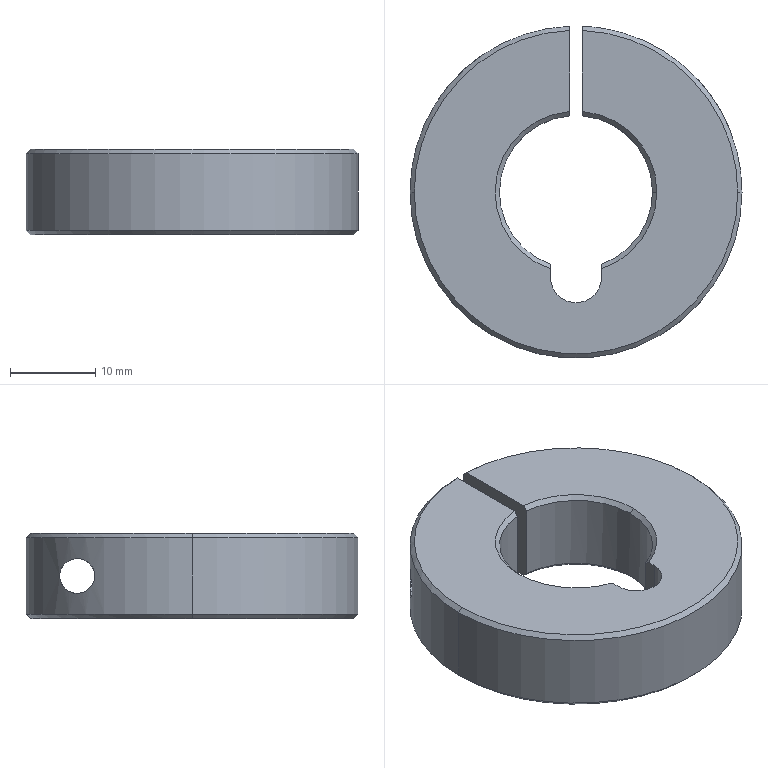Part | SolidWorks | features BaseBody 1 | 1 solid | 40 faces | box 39 x 38.986 x 10 mm | volume 8129 mm3 | cone 16 | cylinder 15 | plane 9 | commonest cylinder face diameters 5.5 x4 39 x4 18 x3 4.1 x2 6 x1 9 x1
STEP:
#1=CARTESIAN_POINT('',(5.,13.5,-2.75));
#2=VERTEX_POINT('',#1);
#3=CARTESIAN_POINT('',(5.,13.5,2.75));
#4=VERTEX_POINT('',#3);
#5=CARTESIAN_POINT('',(5.,13.5,0.));
#6=DIRECTION('',(-1.,0.,0.));
#7=DIRECTION('',(0.,0.,1.));
#8=AXIS2_PLACEMENT_3D('',#5,#6,#7);
#9=CIRCLE('',#8,2.75);
#10=EDGE_CURVE('',#2,#4,#9,.T.);
#11=ORIENTED_EDGE('',*,*,#10,.T.);
#12=CARTESIAN_POINT('',(5.5,13.5,3.25));
#13=VERTEX_POINT('',#12);
#14=CARTESIAN_POINT('',(5.5,13.5,3.25));
#15=DIRECTION('',(0.7071,0.,0.7071));
#16=VECTOR('',#15,1000.);
#17=LINE('',#14,#16);
#18=EDGE_CURVE('',#4,#13,#17,.T.);
#19=ORIENTED_EDGE('',*,*,#18,.T.);
#20=CARTESIAN_POINT('',(5.5,13.5,-3.25));
#21=VERTEX_POINT('',#20);
#22=CARTESIAN_POINT('',(5.5,13.5,0.));
#23=DIRECTION('',(-1.,0.,0.));
#24=DIRECTION('',(0.,0.,1.));
#25=AXIS2_PLACEMENT_3D('',#22,#23,#24);
#26=CIRCLE('',#25,3.25);
#27=EDGE_CURVE('',#21,#13,#26,.T.);
#28=ORIENTED_EDGE('',*,*,#27,.F.);
#29=CARTESIAN_POINT('',(5.5,13.5,-3.25));
#30=DIRECTION('',(0.7071,0.,-0.7071));
#31=VECTOR('',#30,1000.);
#32=LINE('',#29,#31);
#33=EDGE_CURVE('',#2,#21,#32,.T.);
#34=ORIENTED_EDGE('',*,*,#33,.F.);
#35=EDGE_LOOP('',(#11,#19,#28,#34));
#36=FACE_OUTER_BOUND('',#35,.T.);
#37=CARTESIAN_POINT('',(5.5,13.5,0.));
#38=DIRECTION('',(1.,0.,0.));
#39=DIRECTION('',(0.,0.,-1.));
#40=AXIS2_PLACEMENT_3D('',#37,#38,#39);
#41=CONICAL_SURFACE('',#40,3.25,0.7854);
#42=ADVANCED_FACE('',(#36),#41,.F.);
#43=ORIENTED_EDGE('',*,*,#10,.F.);
#44=CARTESIAN_POINT('',(0.75,13.5,-2.75));
#45=VERTEX_POINT('',#44);
#46=CARTESIAN_POINT('',(-35.723,13.5,-2.75));
#47=DIRECTION('',(-1.,0.,0.));
#48=VECTOR('',#47,1000.);
#49=LINE('',#46,#48);
#50=EDGE_CURVE('',#2,#45,#49,.T.);
#51=ORIENTED_EDGE('',*,*,#50,.T.);
#52=CARTESIAN_POINT('',(0.75,13.5,2.75));
#53=VERTEX_POINT('',#52);
#54=CARTESIAN_POINT('',(0.75,13.5,0.));
#55=DIRECTION('',(-1.,0.,0.));
#56=DIRECTION('',(0.,0.,-1.));
#57=AXIS2_PLACEMENT_3D('',#54,#55,#56);
#58=CIRCLE('',#57,2.75);
#59=EDGE_CURVE('',#45,#53,#58,.T.);
#60=ORIENTED_EDGE('',*,*,#59,.T.);
#61=CARTESIAN_POINT('',(-35.723,13.5,2.75));
#62=DIRECTION('',(-1.,0.,0.));
#63=VECTOR('',#62,1000.);
#64=LINE('',#61,#63);
#65=EDGE_CURVE('',#4,#53,#64,.T.);
#66=ORIENTED_EDGE('',*,*,#65,.F.);
#67=EDGE_LOOP('',(#43,#51,#60,#66));
#68=FACE_OUTER_BOUND('',#67,.T.);
#69=CARTESIAN_POINT('',(-35.723,13.5,0.));
#70=DIRECTION('',(-1.,0.,0.));
#71=DIRECTION('',(0.,0.,1.));
#72=AXIS2_PLACEMENT_3D('',#69,#70,#71);
#73=CYLINDRICAL_SURFACE('',#72,2.75);
#74=ADVANCED_FACE('',(#68),#73,.F.);
#75=CARTESIAN_POINT('',(-0.75,13.5,2.75));
#76=VERTEX_POINT('',#75);
#77=CARTESIAN_POINT('',(-0.75,13.5,-2.75));
#78=VERTEX_POINT('',#77);
#79=CARTESIAN_POINT('',(-0.75,13.5,0.));
#80=DIRECTION('',(1.,0.,0.));
#81=DIRECTION('',(0.,0.,1.));
#82=AXIS2_PLACEMENT_3D('',#79,#80,#81);
#83=CIRCLE('',#82,2.75);
#84=EDGE_CURVE('',#76,#78,#83,.T.);
#85=ORIENTED_EDGE('',*,*,#84,.T.);
#86=CARTESIAN_POINT('',(-1.25,13.5,-2.75));
#87=VERTEX_POINT('',#86);
#88=CARTESIAN_POINT('',(-35.723,13.5,-2.75));
#89=DIRECTION('',(-1.,0.,0.));
#90=VECTOR('',#89,1000.);
#91=LINE('',#88,#90);
#92=EDGE_CURVE('',#78,#87,#91,.T.);
#93=ORIENTED_EDGE('',*,*,#92,.T.);
#94=CARTESIAN_POINT('',(-1.25,13.5,2.75));
#95=VERTEX_POINT('',#94);
#96=CARTESIAN_POINT('',(-1.25,13.5,0.));
#97=DIRECTION('',(-1.,0.,0.));
#98=DIRECTION('',(0.,0.,1.));
#99=AXIS2_PLACEMENT_3D('',#96,#97,#98);
#100=CIRCLE('',#99,2.75);
#101=EDGE_CURVE('',#87,#95,#100,.T.);
#102=ORIENTED_EDGE('',*,*,#101,.T.);
#103=CARTESIAN_POINT('',(-35.723,13.5,2.75));
#104=DIRECTION('',(-1.,0.,0.));
#105=VECTOR('',#104,1000.);
#106=LINE('',#103,#105);
#107=EDGE_CURVE('',#76,#95,#106,.T.);
#108=ORIENTED_EDGE('',*,*,#107,.F.);
#109=EDGE_LOOP('',(#85,#93,#102,#108));
#110=FACE_OUTER_BOUND('',#109,.T.);
#111=CARTESIAN_POINT('',(-35.723,13.5,0.));
#112=DIRECTION('',(-1.,0.,0.));
#113=DIRECTION('',(0.,0.,1.));
#114=AXIS2_PLACEMENT_3D('',#111,#112,#113);
#115=CYLINDRICAL_SURFACE('',#114,2.75);
#116=ADVANCED_FACE('',(#110),#115,.F.);
#117=CARTESIAN_POINT('',(-1.654,13.5,-2.05));
#118=VERTEX_POINT('',#117);
#119=CARTESIAN_POINT('',(-1.654,13.5,2.05));
#120=VERTEX_POINT('',#119);
#121=CARTESIAN_POINT('',(-1.654,13.5,0.));
#122=DIRECTION('',(-1.,0.,0.));
#123=DIRECTION('',(0.,0.,1.));
#124=AXIS2_PLACEMENT_3D('',#121,#122,#123);
#125=CIRCLE('',#124,2.05);
#126=EDGE_CURVE('',#118,#120,#125,.T.);
#127=ORIENTED_EDGE('',*,*,#126,.T.);
#128=CARTESIAN_POINT('',(-1.25,13.5,2.75));
#129=DIRECTION('',(0.5,0.,0.866));
#130=VECTOR('',#129,1000.);
#131=LINE('',#128,#130);
#132=EDGE_CURVE('',#120,#95,#131,.T.);
#133=ORIENTED_EDGE('',*,*,#132,.T.);
#134=ORIENTED_EDGE('',*,*,#101,.F.);
#135=CARTESIAN_POINT('',(-1.25,13.5,-2.75));
#136=DIRECTION('',(0.5,0.,-0.866));
#137=VECTOR('',#136,1000.);
#138=LINE('',#135,#137);
#139=EDGE_CURVE('',#118,#87,#138,.T.);
#140=ORIENTED_EDGE('',*,*,#139,.F.);
#141=EDGE_LOOP('',(#127,#133,#134,#140));
#142=FACE_OUTER_BOUND('',#141,.T.);
#143=CARTESIAN_POINT('',(-1.25,13.5,0.));
#144=DIRECTION('',(1.,0.,0.));
#145=DIRECTION('',(0.,0.,-1.));
#146=AXIS2_PLACEMENT_3D('',#143,#144,#145);
#147=CONICAL_SURFACE('',#146,2.75,1.047);
#148=ADVANCED_FACE('',(#142),#147,.F.);
#149=ORIENTED_EDGE('',*,*,#126,.F.);
#150=CARTESIAN_POINT('',(-14.071,13.5,-2.05));
#151=VERTEX_POINT('',#150);
#152=CARTESIAN_POINT('',(-35.723,13.5,-2.05));
#153=DIRECTION('',(-1.,0.,0.));
#154=VECTOR('',#153,1000.);
#155=LINE('',#152,#154);
#156=EDGE_CURVE('',#118,#151,#155,.T.);
#157=ORIENTED_EDGE('',*,*,#156,.T.);
#158=CARTESIAN_POINT('',(-14.071,13.5,2.05));
#159=VERTEX_POINT('',#158);
#160=CARTESIAN_POINT('',(-14.071,13.5,-2.05));
#161=CARTESIAN_POINT('',(-14.193,13.374,-2.05));
#162=CARTESIAN_POINT('',(-14.305,13.253,-2.038));
#163=CARTESIAN_POINT('',(-14.461,13.082,-2.008));
#164=CARTESIAN_POINT('',(-14.51,13.027,-1.995));
#165=CARTESIAN_POINT('',(-14.581,12.947,-1.974));
#166=CARTESIAN_POINT('',(-14.616,12.908,-1.963));
#167=CARTESIAN_POINT('',(-14.655,12.864,-1.949));
#168=CARTESIAN_POINT('',(-14.672,12.845,-1.942));
#169=CARTESIAN_POINT('',(-14.683,12.832,-1.938));
#170=CARTESIAN_POINT('',(-14.687,12.828,-1.937));
#171=CARTESIAN_POINT('',(-14.801,12.696,-1.89));
#172=CARTESIAN_POINT('',(-14.901,12.579,-1.836));
#173=CARTESIAN_POINT('',(-15.037,12.415,-1.741));
#174=CARTESIAN_POINT('',(-15.08,12.363,-1.707));
#175=CARTESIAN_POINT('',(-15.142,12.287,-1.653));
#176=CARTESIAN_POINT('',(-15.172,12.25,-1.625));
#177=CARTESIAN_POINT('',(-15.205,12.208,-1.592));
#178=CARTESIAN_POINT('',(-15.219,12.191,-1.578));
#179=CARTESIAN_POINT('',(-15.229,12.179,-1.568));
#180=CARTESIAN_POINT('',(-15.233,12.174,-1.564));
#181=CARTESIAN_POINT('',(-15.325,12.059,-1.465));
#182=CARTESIAN_POINT('',(-15.401,11.961,-1.361));
#183=CARTESIAN_POINT('',(-15.5,11.832,-1.194));
#184=CARTESIAN_POINT('',(-15.531,11.792,-1.136));
#185=CARTESIAN_POINT('',(-15.572,11.737,-1.046));
#186=CARTESIAN_POINT('',(-15.592,11.71,-1.001));
#187=CARTESIAN_POINT('',(-15.611,11.686,-0.955));
#188=CARTESIAN_POINT('',(-15.622,11.67,-0.9241));
#189=CARTESIAN_POINT('',(-15.628,11.663,-0.9102));
#190=CARTESIAN_POINT('',(-15.734,11.521,-0.6165));
#191=CARTESIAN_POINT('',(-15.784,11.451,-0.3117));
#192=CARTESIAN_POINT('',(-15.785,11.45,0.1475));
#193=CARTESIAN_POINT('',(-15.773,11.466,0.3009));
#194=CARTESIAN_POINT('',(-15.736,11.517,0.5257));
#195=CARTESIAN_POINT('',(-15.72,11.538,0.5998));
#196=CARTESIAN_POINT('',(-15.692,11.576,0.7088));
#197=CARTESIAN_POINT('',(-15.677,11.597,0.7628));
#198=CARTESIAN_POINT('',(-15.66,11.619,0.8159));
#199=CARTESIAN_POINT('',(-15.649,11.635,0.8511));
#200=CARTESIAN_POINT('',(-15.642,11.644,0.8703));
#201=CARTESIAN_POINT('',(-15.592,11.711,1.011));
#202=CARTESIAN_POINT('',(-15.536,11.785,1.132));
#203=CARTESIAN_POINT('',(-15.438,11.914,1.3));
#204=CARTESIAN_POINT('',(-15.402,11.96,1.354));
#205=CARTESIAN_POINT('',(-15.345,12.033,1.432));
#206=CARTESIAN_POINT('',(-15.315,12.071,1.47));
#207=CARTESIAN_POINT('',(-15.279,12.116,1.513));
#208=CARTESIAN_POINT('',(-15.263,12.136,1.531));
#209=CARTESIAN_POINT('',(-15.252,12.15,1.543));
#210=CARTESIAN_POINT('',(-15.246,12.158,1.549));
#211=CARTESIAN_POINT('',(-15.168,12.255,1.634));
#212=CARTESIAN_POINT('',(-15.086,12.357,1.706));
#213=CARTESIAN_POINT('',(-14.95,12.52,1.802));
#214=CARTESIAN_POINT('',(-14.902,12.577,1.831));
#215=CARTESIAN_POINT('',(-14.828,12.664,1.872));
#216=CARTESIAN_POINT('',(-14.79,12.709,1.892));
#217=CARTESIAN_POINT('',(-14.744,12.762,1.913));
#218=CARTESIAN_POINT('',(-14.724,12.785,1.921));
#219=CARTESIAN_POINT('',(-14.711,12.8,1.927));
#220=CARTESIAN_POINT('',(-14.702,12.81,1.93));
#221=CARTESIAN_POINT('',(-14.524,13.014,2.003));
#222=CARTESIAN_POINT('',(-14.315,13.245,2.05));
#223=CARTESIAN_POINT('',(-14.071,13.5,2.05));
#224=B_SPLINE_CURVE_WITH_KNOTS('',3,(#160,#161,#162,#163,#164,#165,#166,#167,#168,#169,#170,#171,#172,#173,#174,#175,#176,#177,#178,#179,#180,#181,#182,#183,#184,#185,#186,#187,#188,#189,#190,#191,#192,#193,#194,#195,#196,#197,#198,#199,#200,#201,#202,#203,#204,#205,#206,#207,#208,#209,#210,#211,#212,#213,#214,#215,#216,#217,#218,#219,#220,#221,#222,#223),.UNSPECIFIED.,.F.,.F.,(4,2,2,1,1,2,2,2,2,1,1,2,2,2,2,1,2,2,2,2,2,1,2,2,2,2,1,1,2,2,2,2,1,1,2,2,4),(0.,0.0625,0.09375,0.1094,0.1172,0.1211,0.125,0.1875,0.2187,0.2344,0.2422,0.2461,0.25,0.3125,0.3437,0.3594,0.3672,0.375,0.5,0.5625,0.5937,0.6094,0.6172,0.625,0.6875,0.7187,0.7344,0.7422,0.7461,0.75,0.8125,0.8437,0.8594,0.8672,0.8711,0.875,1.),.UNSPECIFIED.);
#225=EDGE_CURVE('',#151,#159,#224,.T.);
#226=ORIENTED_EDGE('',*,*,#225,.T.);
#227=CARTESIAN_POINT('',(-35.723,13.5,2.05));
#228=DIRECTION('',(-1.,0.,0.));
#229=VECTOR('',#228,1000.);
#230=LINE('',#227,#229);
#231=EDGE_CURVE('',#120,#159,#230,.T.);
#232=ORIENTED_EDGE('',*,*,#231,.F.);
#233=EDGE_LOOP('',(#149,#157,#226,#232));
#234=FACE_OUTER_BOUND('',#233,.T.);
#235=CARTESIAN_POINT('',(-35.723,13.5,0.));
#236=DIRECTION('',(-1.,0.,0.));
#237=DIRECTION('',(0.,0.,1.));
#238=AXIS2_PLACEMENT_3D('',#235,#236,#237);
#239=CYLINDRICAL_SURFACE('',#238,2.05);
#240=ADVANCED_FACE('',(#234),#239,.F.);
#241=CARTESIAN_POINT('',(19.,0.,5.));
#242=VERTEX_POINT('',#241);
#243=CARTESIAN_POINT('',(0.75,18.985,5.));
#244=VERTEX_POINT('',#243);
#245=CARTESIAN_POINT('',(0.,0.,5.));
#246=DIRECTION('',(0.,0.,1.));
#247=DIRECTION('',(1.,0.,0.));
#248=AXIS2_PLACEMENT_3D('',#245,#246,#247);
#249=CIRCLE('',#248,19.);
#250=EDGE_CURVE('',#242,#244,#249,.T.);
#251=ORIENTED_EDGE('',*,*,#250,.F.);
#252=CARTESIAN_POINT('',(19.5,0.,4.5));
#253=VERTEX_POINT('',#252);
#254=CARTESIAN_POINT('',(19.,0.,5.));
#255=DIRECTION('',(0.7071,0.,-0.7071));
#256=VECTOR('',#255,1000.);
#257=LINE('',#254,#256);
#258=EDGE_CURVE('',#242,#253,#257,.T.);
#259=ORIENTED_EDGE('',*,*,#258,.T.);
#260=CARTESIAN_POINT('',(14.071,13.5,4.5));
#261=VERTEX_POINT('',#260);
#262=CARTESIAN_POINT('',(0.,0.,4.5));
#263=DIRECTION('',(0.,0.,-1.));
#264=DIRECTION('',(1.,0.,0.));
#265=AXIS2_PLACEMENT_3D('',#262,#263,#264);
#266=CIRCLE('',#265,19.5);
#267=EDGE_CURVE('',#261,#253,#266,.T.);
#268=ORIENTED_EDGE('',*,*,#267,.F.);
#269=CARTESIAN_POINT('',(5.5,18.708,4.5));
#270=VERTEX_POINT('',#269);
#271=CARTESIAN_POINT('',(0.,0.,4.5));
#272=DIRECTION('',(0.,0.,1.));
#273=DIRECTION('',(0.,1.,0.));
#274=AXIS2_PLACEMENT_3D('',#271,#272,#273);
#275=CIRCLE('',#274,19.5);
#276=EDGE_CURVE('',#261,#270,#275,.T.);
#277=ORIENTED_EDGE('',*,*,#276,.T.);
#278=CARTESIAN_POINT('',(0.75,19.486,4.5));
#279=VERTEX_POINT('',#278);
#280=CARTESIAN_POINT('',(0.,0.,4.5));
#281=DIRECTION('',(0.,0.,-1.));
#282=DIRECTION('',(1.,0.,0.));
#283=AXIS2_PLACEMENT_3D('',#280,#281,#282);
#284=CIRCLE('',#283,19.5);
#285=EDGE_CURVE('',#279,#270,#284,.T.);
#286=ORIENTED_EDGE('',*,*,#285,.F.);
#287=CARTESIAN_POINT('',(0.75,18.985,5.));
#288=CARTESIAN_POINT('',(0.75,19.152,4.833));
#289=CARTESIAN_POINT('',(0.75,19.319,4.667));
#290=CARTESIAN_POINT('',(0.75,19.486,4.5));
#291=B_SPLINE_CURVE_WITH_KNOTS('',3,(#287,#288,#289,#290),.UNSPECIFIED.,.F.,.F.,(4,4),(0.,0.0007074),.UNSPECIFIED.);
#292=EDGE_CURVE('',#244,#279,#291,.T.);
#293=ORIENTED_EDGE('',*,*,#292,.F.);
#294=EDGE_LOOP('',(#251,#259,#268,#277,#286,#293));
#295=FACE_OUTER_BOUND('',#294,.T.);
#296=CARTESIAN_POINT('',(0.,0.,5.));
#297=DIRECTION('',(0.,0.,-1.));
#298=DIRECTION('',(-1.,0.,0.));
#299=AXIS2_PLACEMENT_3D('',#296,#297,#298);
#300=CONICAL_SURFACE('',#299,19.,0.7854);
#301=ADVANCED_FACE('',(#295),#300,.T.);
#302=ORIENTED_EDGE('',*,*,#258,.F.);
#303=CARTESIAN_POINT('',(-19.,0.,5.));
#304=VERTEX_POINT('',#303);
#305=CARTESIAN_POINT('',(0.,0.,5.));
#306=DIRECTION('',(0.,0.,1.));
#307=DIRECTION('',(1.,0.,0.));
#308=AXIS2_PLACEMENT_3D('',#305,#306,#307);
#309=CIRCLE('',#308,19.);
#310=EDGE_CURVE('',#304,#242,#309,.T.);
#311=ORIENTED_EDGE('',*,*,#310,.F.);
#312=CARTESIAN_POINT('',(-19.5,0.,4.5));
#313=VERTEX_POINT('',#312);
#314=CARTESIAN_POINT('',(-19.,0.,5.));
#315=DIRECTION('',(-0.7071,0.,-0.7071));
#316=VECTOR('',#315,1000.);
#317=LINE('',#314,#316);
#318=EDGE_CURVE('',#304,#313,#317,.T.);
#319=ORIENTED_EDGE('',*,*,#318,.T.);
#320=CARTESIAN_POINT('',(0.,0.,4.5));
#321=DIRECTION('',(0.,0.,-1.));
#322=DIRECTION('',(1.,0.,0.));
#323=AXIS2_PLACEMENT_3D('',#320,#321,#322);
#324=CIRCLE('',#323,19.5);
#325=EDGE_CURVE('',#253,#313,#324,.T.);
#326=ORIENTED_EDGE('',*,*,#325,.F.);
#327=EDGE_LOOP('',(#302,#311,#319,#326));
#328=FACE_OUTER_BOUND('',#327,.T.);
#329=CARTESIAN_POINT('',(0.,0.,5.));
#330=DIRECTION('',(0.,0.,-1.));
#331=DIRECTION('',(-1.,0.,0.));
#332=AXIS2_PLACEMENT_3D('',#329,#330,#331);
#333=CONICAL_SURFACE('',#332,19.,0.7854);
#334=ADVANCED_FACE('',(#328),#333,.T.);
#335=CARTESIAN_POINT('',(-19.,0.,-5.));
#336=VERTEX_POINT('',#335);
#337=CARTESIAN_POINT('',(-0.75,18.985,-5.));
#338=VERTEX_POINT('',#337);
#339=CARTESIAN_POINT('',(0.,0.,-5.));
#340=DIRECTION('',(0.,0.,-1.));
#341=DIRECTION('',(1.,0.,0.));
#342=AXIS2_PLACEMENT_3D('',#339,#340,#341);
#343=CIRCLE('',#342,19.);
#344=EDGE_CURVE('',#336,#338,#343,.T.);
#345=ORIENTED_EDGE('',*,*,#344,.F.);
#346=CARTESIAN_POINT('',(-19.5,0.,-4.5));
#347=VERTEX_POINT('',#346);
#348=CARTESIAN_POINT('',(-19.5,0.,-4.5));
#349=DIRECTION('',(-0.7071,0.,0.7071));
#350=VECTOR('',#349,1000.);
#351=LINE('',#348,#350);
#352=EDGE_CURVE('',#336,#347,#351,.T.);
#353=ORIENTED_EDGE('',*,*,#352,.T.);
#354=CARTESIAN_POINT('',(-0.75,19.486,-4.5));
#355=VERTEX_POINT('',#354);
#356=CARTESIAN_POINT('',(0.,0.,-4.5));
#357=DIRECTION('',(0.,0.,1.));
#358=DIRECTION('',(1.,0.,0.));
#359=AXIS2_PLACEMENT_3D('',#356,#357,#358);
#360=CIRCLE('',#359,19.5);
#361=EDGE_CURVE('',#355,#347,#360,.T.);
#362=ORIENTED_EDGE('',*,*,#361,.F.);
#363=CARTESIAN_POINT('',(-0.75,18.985,-5.));
#364=CARTESIAN_POINT('',(-0.75,19.152,-4.833));
#365=CARTESIAN_POINT('',(-0.75,19.319,-4.667));
#366=CARTESIAN_POINT('',(-0.75,19.486,-4.5));
#367=B_SPLINE_CURVE_WITH_KNOTS('',3,(#363,#364,#365,#366),.UNSPECIFIED.,.F.,.F.,(4,4),(0.,0.0007074),.UNSPECIFIED.);
#368=EDGE_CURVE('',#338,#355,#367,.T.);
#369=ORIENTED_EDGE('',*,*,#368,.F.);
#370=EDGE_LOOP('',(#345,#353,#362,#369));
#371=FACE_OUTER_BOUND('',#370,.T.);
#372=CARTESIAN_POINT('',(0.,0.,-4.5));
#373=DIRECTION('',(0.,0.,1.));
#374=DIRECTION('',(1.,0.,0.));
#375=AXIS2_PLACEMENT_3D('',#372,#373,#374);
#376=CONICAL_SURFACE('',#375,19.5,0.7854);
#377=ADVANCED_FACE('',(#371),#376,.T.);
#378=ORIENTED_EDGE('',*,*,#352,.F.);
#379=CARTESIAN_POINT('',(19.,0.,-5.));
#380=VERTEX_POINT('',#379);
#381=CARTESIAN_POINT('',(0.,0.,-5.));
#382=DIRECTION('',(0.,0.,-1.));
#383=DIRECTION('',(1.,0.,0.));
#384=AXIS2_PLACEMENT_3D('',#381,#382,#383);
#385=CIRCLE('',#384,19.);
#386=EDGE_CURVE('',#380,#336,#385,.T.);
#387=ORIENTED_EDGE('',*,*,#386,.F.);
#388=CARTESIAN_POINT('',(19.5,0.,-4.5));
#389=VERTEX_POINT('',#388);
#390=CARTESIAN_POINT('',(19.5,0.,-4.5));
#391=DIRECTION('',(0.7071,0.,0.7071));
#392=VECTOR('',#391,1000.);
#393=LINE('',#390,#392);
#394=EDGE_CURVE('',#380,#389,#393,.T.);
#395=ORIENTED_EDGE('',*,*,#394,.T.);
#396=CARTESIAN_POINT('',(0.,0.,-4.5));
#397=DIRECTION('',(0.,0.,1.));
#398=DIRECTION('',(1.,0.,0.));
#399=AXIS2_PLACEMENT_3D('',#396,#397,#398);
#400=CIRCLE('',#399,19.5);
#401=EDGE_CURVE('',#347,#389,#400,.T.);
#402=ORIENTED_EDGE('',*,*,#401,.F.);
#403=EDGE_LOOP('',(#378,#387,#395,#402));
#404=FACE_OUTER_BOUND('',#403,.T.);
#405=CARTESIAN_POINT('',(0.,0.,-4.5));
#406=DIRECTION('',(0.,0.,1.));
#407=DIRECTION('',(1.,0.,0.));
#408=AXIS2_PLACEMENT_3D('',#405,#406,#407);
#409=CONICAL_SURFACE('',#408,19.5,0.7854);
#410=ADVANCED_FACE('',(#404),#409,.T.);
#411=CARTESIAN_POINT('',(-9.,0.,-4.5));
#412=VERTEX_POINT('',#411);
#413=CARTESIAN_POINT('',(-0.75,8.969,-4.5));
#414=VERTEX_POINT('',#413);
#415=CARTESIAN_POINT('',(0.,0.,-4.5));
#416=DIRECTION('',(0.,0.,-1.));
#417=DIRECTION('',(1.,0.,0.));
#418=AXIS2_PLACEMENT_3D('',#415,#416,#417);
#419=CIRCLE('',#418,9.);
#420=EDGE_CURVE('',#412,#414,#419,.T.);
#421=ORIENTED_EDGE('',*,*,#420,.F.);
#422=CARTESIAN_POINT('',(-9.5,0.,-5.));
#423=VERTEX_POINT('',#422);
#424=CARTESIAN_POINT('',(-9.,0.,-4.5));
#425=DIRECTION('',(-0.7071,0.,-0.7071));
#426=VECTOR('',#425,1000.);
#427=LINE('',#424,#426);
#428=EDGE_CURVE('',#412,#423,#427,.T.);
#429=ORIENTED_EDGE('',*,*,#428,.T.);
#430=CARTESIAN_POINT('',(-0.75,9.47,-5.));
#431=VERTEX_POINT('',#430);
#432=CARTESIAN_POINT('',(0.,0.,-5.));
#433=DIRECTION('',(0.,0.,1.));
#434=DIRECTION('',(1.,0.,0.));
#435=AXIS2_PLACEMENT_3D('',#432,#433,#434);
#436=CIRCLE('',#435,9.5);
#437=EDGE_CURVE('',#431,#423,#436,.T.);
#438=ORIENTED_EDGE('',*,*,#437,.F.);
#439=CARTESIAN_POINT('',(-0.75,8.969,-4.5));
#440=CARTESIAN_POINT('',(-0.75,9.136,-4.667));
#441=CARTESIAN_POINT('',(-0.75,9.303,-4.833));
#442=CARTESIAN_POINT('',(-0.75,9.47,-5.));
#443=B_SPLINE_CURVE_WITH_KNOTS('',3,(#439,#440,#441,#442),.UNSPECIFIED.,.F.,.F.,(4,4),(0.,0.0007083),.UNSPECIFIED.);
#444=EDGE_CURVE('',#414,#431,#443,.T.);
#445=ORIENTED_EDGE('',*,*,#444,.F.);
#446=EDGE_LOOP('',(#421,#429,#438,#445));
#447=FACE_OUTER_BOUND('',#446,.T.);
#448=CARTESIAN_POINT('',(0.,0.,-4.5));
#449=DIRECTION('',(0.,0.,-1.));
#450=DIRECTION('',(-1.,0.,0.));
#451=AXIS2_PLACEMENT_3D('',#448,#449,#450);
#452=CONICAL_SURFACE('',#451,9.,0.7854);
#453=ADVANCED_FACE('',(#447),#452,.F.);
#454=CARTESIAN_POINT('',(9.,0.,4.5));
#455=VERTEX_POINT('',#454);
#456=CARTESIAN_POINT('',(0.75,8.969,4.5));
#457=VERTEX_POINT('',#456);
#458=CARTESIAN_POINT('',(0.,0.,4.5));
#459=DIRECTION('',(0.,0.,1.));
#460=DIRECTION('',(1.,0.,0.));
#461=AXIS2_PLACEMENT_3D('',#458,#459,#460);
#462=CIRCLE('',#461,9.);
#463=EDGE_CURVE('',#455,#457,#462,.T.);
#464=ORIENTED_EDGE('',*,*,#463,.F.);
#465=CARTESIAN_POINT('',(9.5,0.,5.));
#466=VERTEX_POINT('',#465);
#467=CARTESIAN_POINT('',(9.5,0.,5.));
#468=DIRECTION('',(0.7071,0.,0.7071));
#469=VECTOR('',#468,1000.);
#470=LINE('',#467,#469);
#471=EDGE_CURVE('',#455,#466,#470,.T.);
#472=ORIENTED_EDGE('',*,*,#471,.T.);
#473=CARTESIAN_POINT('',(0.75,9.47,5.));
#474=VERTEX_POINT('',#473);
#475=CARTESIAN_POINT('',(0.,0.,5.));
#476=DIRECTION('',(0.,0.,-1.));
#477=DIRECTION('',(1.,0.,0.));
#478=AXIS2_PLACEMENT_3D('',#475,#476,#477);
#479=CIRCLE('',#478,9.5);
#480=EDGE_CURVE('',#474,#466,#479,.T.);
#481=ORIENTED_EDGE('',*,*,#480,.F.);
#482=CARTESIAN_POINT('',(0.75,8.969,4.5));
#483=CARTESIAN_POINT('',(0.75,9.136,4.667));
#484=CARTESIAN_POINT('',(0.75,9.303,4.833));
#485=CARTESIAN_POINT('',(0.75,9.47,5.));
#486=B_SPLINE_CURVE_WITH_KNOTS('',3,(#482,#483,#484,#485),.UNSPECIFIED.,.F.,.F.,(4,4),(0.,0.0007083),.UNSPECIFIED.);
#487=EDGE_CURVE('',#457,#474,#486,.T.);
#488=ORIENTED_EDGE('',*,*,#487,.F.);
#489=EDGE_LOOP('',(#464,#472,#481,#488));
#490=FACE_OUTER_BOUND('',#489,.T.);
#491=CARTESIAN_POINT('',(0.,0.,5.));
#492=DIRECTION('',(0.,0.,1.));
#493=DIRECTION('',(1.,0.,0.));
#494=AXIS2_PLACEMENT_3D('',#491,#492,#493);
#495=CONICAL_SURFACE('',#494,9.5,0.7854);
#496=ADVANCED_FACE('',(#490),#495,.F.);
#497=CARTESIAN_POINT('',(-0.75,8.969,4.5));
#498=VERTEX_POINT('',#497);
#499=CARTESIAN_POINT('',(-9.,0.,4.5));
#500=VERTEX_POINT('',#499);
#501=CARTESIAN_POINT('',(0.,0.,4.5));
#502=DIRECTION('',(0.,0.,1.));
#503=DIRECTION('',(1.,0.,0.));
#504=AXIS2_PLACEMENT_3D('',#501,#502,#503);
#505=CIRCLE('',#504,9.);
#506=EDGE_CURVE('',#498,#500,#505,.T.);
#507=ORIENTED_EDGE('',*,*,#506,.T.);
#508=CARTESIAN_POINT('',(-9.,0.,5.));
#509=DIRECTION('',(0.,0.,-1.));
#510=VECTOR('',#509,1000.);
#511=LINE('',#508,#510);
#512=EDGE_CURVE('',#500,#412,#511,.T.);
#513=ORIENTED_EDGE('',*,*,#512,.T.);
#514=ORIENTED_EDGE('',*,*,#420,.T.);
#515=CARTESIAN_POINT('',(-0.75,8.969,5.));
#516=DIRECTION('',(0.,0.,-1.));
#517=VECTOR('',#516,1000.);
#518=LINE('',#515,#517);
#519=EDGE_CURVE('',#498,#414,#518,.T.);
#520=ORIENTED_EDGE('',*,*,#519,.F.);
#521=EDGE_LOOP('',(#507,#513,#514,#520));
#522=FACE_OUTER_BOUND('',#521,.T.);
#523=CARTESIAN_POINT('',(0.,0.,5.));
#524=DIRECTION('',(0.,0.,-1.));
#525=DIRECTION('',(-1.,0.,0.));
#526=AXIS2_PLACEMENT_3D('',#523,#524,#525);
#527=CYLINDRICAL_SURFACE('',#526,9.);
#528=ADVANCED_FACE('',(#522),#527,.F.);
#529=ORIENTED_EDGE('',*,*,#267,.T.);
#530=CARTESIAN_POINT('',(19.5,0.,5.));
#531=DIRECTION('',(0.,0.,-1.));
#532=VECTOR('',#531,1000.);
#533=LINE('',#530,#532);
#534=EDGE_CURVE('',#253,#389,#533,.T.);
#535=ORIENTED_EDGE('',*,*,#534,.T.);
#536=CARTESIAN_POINT('',(14.071,13.5,-4.5));
#537=VERTEX_POINT('',#536);
#538=CARTESIAN_POINT('',(0.,0.,-4.5));
#539=DIRECTION('',(0.,0.,1.));
#540=DIRECTION('',(1.,0.,0.));
#541=AXIS2_PLACEMENT_3D('',#538,#539,#540);
#542=CIRCLE('',#541,19.5);
#543=EDGE_CURVE('',#389,#537,#542,.T.);
#544=ORIENTED_EDGE('',*,*,#543,.T.);
#545=CARTESIAN_POINT('',(14.071,13.5,4.5));
#546=CARTESIAN_POINT('',(14.587,12.962,4.5));
#547=CARTESIAN_POINT('',(15.039,12.426,4.403));
#548=CARTESIAN_POINT('',(15.62,11.674,4.122));
#549=CARTESIAN_POINT('',(15.798,11.433,4.006));
#550=CARTESIAN_POINT('',(16.04,11.088,3.802));
#551=CARTESIAN_POINT('',(16.117,10.977,3.728));
#552=CARTESIAN_POINT('',(16.226,10.815,3.611));
#553=CARTESIAN_POINT('',(16.279,10.735,3.551));
#554=CARTESIAN_POINT('',(16.339,10.644,3.478));
#555=CARTESIAN_POINT('',(16.368,10.599,3.441));
#556=CARTESIAN_POINT('',(16.38,10.58,3.424));
#557=CARTESIAN_POINT('',(16.388,10.568,3.414));
#558=CARTESIAN_POINT('',(16.392,10.562,3.409));
#559=CARTESIAN_POINT('',(16.696,10.089,2.999));
#560=CARTESIAN_POINT('',(16.921,9.697,2.49));
#561=CARTESIAN_POINT('',(17.222,9.153,1.329));
#562=CARTESIAN_POINT('',(17.298,9.002,0.6796));
#563=CARTESIAN_POINT('',(17.3,8.998,-0.6571));
#564=CARTESIAN_POINT('',(17.225,9.148,-1.312));
#565=CARTESIAN_POINT('',(17.001,9.554,-2.187));
#566=CARTESIAN_POINT('',(16.907,9.72,-2.462));
#567=CARTESIAN_POINT('',(16.738,10.005,-2.839));
#568=CARTESIAN_POINT('',(16.677,10.106,-2.959));
#569=CARTESIAN_POINT('',(16.579,10.266,-3.131));
#570=CARTESIAN_POINT('',(16.528,10.348,-3.214));
#571=CARTESIAN_POINT('',(16.465,10.448,-3.307));
#572=CARTESIAN_POINT('',(16.433,10.498,-3.352));
#573=CARTESIAN_POINT('',(16.419,10.52,-3.371));
#574=CARTESIAN_POINT('',(16.41,10.534,-3.384));
#575=CARTESIAN_POINT('',(16.405,10.542,-3.391));
#576=CARTESIAN_POINT('',(16.141,10.952,-3.747));
#577=CARTESIAN_POINT('',(15.818,11.419,-4.026));
#578=CARTESIAN_POINT('',(15.041,12.423,-4.402));
#579=CARTESIAN_POINT('',(14.588,12.961,-4.5));
#580=CARTESIAN_POINT('',(14.071,13.5,-4.5));
#581=B_SPLINE_CURVE_WITH_KNOTS('',3,(#545,#546,#547,#548,#549,#550,#551,#552,#553,#554,#555,#556,#557,#558,#559,#560,#561,#562,#563,#564,#565,#566,#567,#568,#569,#570,#571,#572,#573,#574,#575,#576,#577,#578,#579,#580),.UNSPECIFIED.,.F.,.F.,(4,2,2,2,1,1,1,2,2,2,2,2,2,2,1,1,1,2,2,2,4),(0.,0.125,0.1875,0.2187,0.2344,0.2422,0.2461,0.248,0.25,0.375,0.5,0.625,0.6875,0.7187,0.7344,0.7422,0.7461,0.748,0.75,0.875,1.),.UNSPECIFIED.);
#582=EDGE_CURVE('',#261,#537,#581,.T.);
#583=ORIENTED_EDGE('',*,*,#582,.F.);
#584=EDGE_LOOP('',(#529,#535,#544,#583));
#585=FACE_OUTER_BOUND('',#584,.T.);
#586=CARTESIAN_POINT('',(0.,0.,5.));
#587=DIRECTION('',(0.,0.,-1.));
#588=DIRECTION('',(-1.,0.,0.));
#589=AXIS2_PLACEMENT_3D('',#586,#587,#588);
#590=CYLINDRICAL_SURFACE('',#589,19.5);
#591=ADVANCED_FACE('',(#585),#590,.T.);
#592=ORIENTED_EDGE('',*,*,#534,.F.);
#593=ORIENTED_EDGE('',*,*,#325,.T.);
#594=CARTESIAN_POINT('',(-19.5,0.,5.));
#595=DIRECTION('',(0.,0.,-1.));
#596=VECTOR('',#595,1000.);
#597=LINE('',#594,#596);
#598=EDGE_CURVE('',#313,#347,#597,.T.);
#599=ORIENTED_EDGE('',*,*,#598,.T.);
#600=ORIENTED_EDGE('',*,*,#401,.T.);
#601=EDGE_LOOP('',(#592,#593,#599,#600));
#602=FACE_OUTER_BOUND('',#601,.T.);
#603=CARTESIAN_POINT('',(0.,0.,5.));
#604=DIRECTION('',(0.,0.,-1.));
#605=DIRECTION('',(-1.,0.,0.));
#606=AXIS2_PLACEMENT_3D('',#603,#604,#605);
#607=CYLINDRICAL_SURFACE('',#606,19.5);
#608=ADVANCED_FACE('',(#602),#607,.T.);
#609=CARTESIAN_POINT('',(5.5,18.708,-4.5));
#610=VERTEX_POINT('',#609);
#611=CARTESIAN_POINT('',(5.5,18.708,5.));
#612=DIRECTION('',(0.,0.,1.));
#613=VECTOR('',#612,1000.);
#614=LINE('',#611,#613);
#615=EDGE_CURVE('',#610,#270,#614,.T.);
#616=ORIENTED_EDGE('',*,*,#615,.F.);
#617=CARTESIAN_POINT('',(0.75,19.486,-4.5));
#618=VERTEX_POINT('',#617);
#619=CARTESIAN_POINT('',(0.,0.,-4.5));
#620=DIRECTION('',(0.,0.,1.));
#621=DIRECTION('',(1.,0.,0.));
#622=AXIS2_PLACEMENT_3D('',#619,#620,#621);
#623=CIRCLE('',#622,19.5);
#624=EDGE_CURVE('',#610,#618,#623,.T.);
#625=ORIENTED_EDGE('',*,*,#624,.T.);
#626=CARTESIAN_POINT('',(0.75,19.486,5.));
#627=DIRECTION('',(0.,0.,-1.));
#628=VECTOR('',#627,1000.);
#629=LINE('',#626,#628);
#630=EDGE_CURVE('',#279,#618,#629,.T.);
#631=ORIENTED_EDGE('',*,*,#630,.F.);
#632=ORIENTED_EDGE('',*,*,#285,.T.);
#633=EDGE_LOOP('',(#616,#625,#631,#632));
#634=FACE_OUTER_BOUND('',#633,.T.);
#635=CARTESIAN_POINT('',(0.,0.,5.));
#636=DIRECTION('',(0.,0.,-1.));
#637=DIRECTION('',(-1.,0.,0.));
#638=AXIS2_PLACEMENT_3D('',#635,#636,#637);
#639=CYLINDRICAL_SURFACE('',#638,19.5);
#640=ADVANCED_FACE('',(#634),#639,.T.);
#641=ORIENTED_EDGE('',*,*,#582,.T.);
#642=CARTESIAN_POINT('',(5.5,13.5,-4.5));
#643=VERTEX_POINT('',#642);
#644=CARTESIAN_POINT('',(19.5,13.5,-4.5));
#645=DIRECTION('',(-1.,0.,0.));
#646=VECTOR('',#645,1000.);
#647=LINE('',#644,#646);
#648=EDGE_CURVE('',#537,#643,#647,.T.);
#649=ORIENTED_EDGE('',*,*,#648,.T.);
#650=CARTESIAN_POINT('',(5.5,13.5,4.5));
#651=VERTEX_POINT('',#650);
#652=CARTESIAN_POINT('',(5.5,13.5,0.));
#653=DIRECTION('',(-1.,0.,0.));
#654=DIRECTION('',(0.,0.,1.));
#655=AXIS2_PLACEMENT_3D('',#652,#653,#654);
#656=CIRCLE('',#655,4.5);
#657=EDGE_CURVE('',#643,#651,#656,.T.);
#658=ORIENTED_EDGE('',*,*,#657,.T.);
#659=CARTESIAN_POINT('',(19.5,13.5,4.5));
#660=DIRECTION('',(-1.,0.,0.));
#661=VECTOR('',#660,1000.);
#662=LINE('',#659,#661);
#663=EDGE_CURVE('',#261,#651,#662,.T.);
#664=ORIENTED_EDGE('',*,*,#663,.F.);
#665=EDGE_LOOP('',(#641,#649,#658,#664));
#666=FACE_OUTER_BOUND('',#665,.T.);
#667=CARTESIAN_POINT('',(-35.723,13.5,0.));
#668=DIRECTION('',(-1.,0.,0.));
#669=DIRECTION('',(0.,0.,1.));
#670=AXIS2_PLACEMENT_3D('',#667,#668,#669);
#671=CYLINDRICAL_SURFACE('',#670,4.5);
#672=ADVANCED_FACE('',(#666),#671,.F.);
#673=CARTESIAN_POINT('',(-14.071,13.5,2.05));
#674=CARTESIAN_POINT('',(-13.997,13.578,2.05));
#675=CARTESIAN_POINT('',(-13.901,13.676,2.046));
#676=CARTESIAN_POINT('',(-13.723,13.854,2.02));
#677=CARTESIAN_POINT('',(-13.659,13.918,2.008));
#678=CARTESIAN_POINT('',(-13.554,14.02,1.983));
#679=CARTESIAN_POINT('',(-13.517,14.055,1.974));
#680=CARTESIAN_POINT('',(-13.461,14.109,1.957));
#681=CARTESIAN_POINT('',(-13.432,14.137,1.949));
#682=CARTESIAN_POINT('',(-13.402,14.165,1.939));
#683=CARTESIAN_POINT('',(-13.382,14.183,1.933));
#684=CARTESIAN_POINT('',(-13.371,14.194,1.929));
#685=CARTESIAN_POINT('',(-13.216,14.339,1.876));
#686=CARTESIAN_POINT('',(-13.084,14.459,1.816));
#687=CARTESIAN_POINT('',(-12.909,14.616,1.721));
#688=CARTESIAN_POINT('',(-12.854,14.664,1.689));
#689=CARTESIAN_POINT('',(-12.778,14.73,1.64));
#690=CARTESIAN_POINT('',(-12.741,14.762,1.616));
#691=CARTESIAN_POINT('',(-12.701,14.797,1.588));
#692=CARTESIAN_POINT('',(-12.681,14.813,1.574));
#693=CARTESIAN_POINT('',(-12.673,14.82,1.568));
#694=CARTESIAN_POINT('',(-12.667,14.825,1.564));
#695=CARTESIAN_POINT('',(-12.666,14.826,1.563));
#696=CARTESIAN_POINT('',(-12.529,14.943,1.463));
#697=CARTESIAN_POINT('',(-12.412,15.041,1.359));
#698=CARTESIAN_POINT('',(-12.26,15.165,1.198));
#699=CARTESIAN_POINT('',(-12.213,15.202,1.144));
#700=CARTESIAN_POINT('',(-12.149,15.253,1.063));
#701=CARTESIAN_POINT('',(-12.119,15.277,1.022));
#702=CARTESIAN_POINT('',(-12.086,15.303,0.9752));
#703=CARTESIAN_POINT('',(-12.07,15.316,0.9516));
#704=CARTESIAN_POINT('',(-12.063,15.321,0.9415));
#705=CARTESIAN_POINT('',(-12.059,15.324,0.9347));
#706=CARTESIAN_POINT('',(-12.057,15.326,0.9327));
#707=CARTESIAN_POINT('',(-11.862,15.479,0.6304));
#708=CARTESIAN_POINT('',(-11.766,15.55,0.3075));
#709=CARTESIAN_POINT('',(-11.766,15.55,-0.1556));
#710=CARTESIAN_POINT('',(-11.791,15.532,-0.3132));
#711=CARTESIAN_POINT('',(-11.863,15.477,-0.5477));
#712=CARTESIAN_POINT('',(-11.893,15.454,-0.6256));
#713=CARTESIAN_POINT('',(-11.947,15.412,-0.741));
#714=CARTESIAN_POINT('',(-11.976,15.389,-0.7983));
#715=CARTESIAN_POINT('',(-12.015,15.359,-0.8644));
#716=CARTESIAN_POINT('',(-12.035,15.343,-0.8972));
#717=CARTESIAN_POINT('',(-12.043,15.336,-0.9112));
#718=CARTESIAN_POINT('',(-12.049,15.332,-0.9205));
#719=CARTESIAN_POINT('',(-12.053,15.329,-0.9264));
#720=CARTESIAN_POINT('',(-12.125,15.272,-1.037));
#721=CARTESIAN_POINT('',(-12.21,15.205,-1.146));
#722=CARTESIAN_POINT('',(-12.362,15.081,-1.306));
#723=CARTESIAN_POINT('',(-12.417,15.036,-1.359));
#724=CARTESIAN_POINT('',(-12.505,14.963,-1.437));
#725=CARTESIAN_POINT('',(-12.55,14.925,-1.475));
#726=CARTESIAN_POINT('',(-12.606,14.878,-1.518));
#727=CARTESIAN_POINT('',(-12.634,14.854,-1.54));
#728=CARTESIAN_POINT('',(-12.649,14.841,-1.55));
#729=CARTESIAN_POINT('',(-12.655,14.836,-1.555));
#730=CARTESIAN_POINT('',(-12.659,14.832,-1.558));
#731=CARTESIAN_POINT('',(-12.662,14.83,-1.56));
#732=CARTESIAN_POINT('',(-12.744,14.76,-1.619));
#733=CARTESIAN_POINT('',(-12.842,14.676,-1.684));
#734=CARTESIAN_POINT('',(-13.017,14.52,-1.779));
#735=CARTESIAN_POINT('',(-13.079,14.464,-1.811));
#736=CARTESIAN_POINT('',(-13.18,14.372,-1.856));
#737=CARTESIAN_POINT('',(-13.232,14.324,-1.878));
#738=CARTESIAN_POINT('',(-13.296,14.264,-1.902));
#739=CARTESIAN_POINT('',(-13.329,14.234,-1.914));
#740=CARTESIAN_POINT('',(-13.343,14.221,-1.919));
#741=CARTESIAN_POINT('',(-13.352,14.212,-1.923));
#742=CARTESIAN_POINT('',(-13.356,14.208,-1.924));
#743=CARTESIAN_POINT('',(-13.544,14.031,-1.989));
#744=CARTESIAN_POINT('',(-13.695,13.881,-2.018));
#745=CARTESIAN_POINT('',(-13.931,13.644,-2.048));
#746=CARTESIAN_POINT('',(-14.017,13.556,-2.05));
#747=CARTESIAN_POINT('',(-14.071,13.5,-2.05));
#748=B_SPLINE_CURVE_WITH_KNOTS('',3,(#673,#674,#675,#676,#677,#678,#679,#680,#681,#682,#683,#684,#685,#686,#687,#688,#689,#690,#691,#692,#693,#694,#695,#696,#697,#698,#699,#700,#701,#702,#703,#704,#705,#706,#707,#708,#709,#710,#711,#712,#713,#714,#715,#716,#717,#718,#719,#720,#721,#722,#723,#724,#725,#726,#727,#728,#729,#730,#731,#732,#733,#734,#735,#736,#737,#738,#739,#740,#741,#742,#743,#744,#745,#746,#747),.UNSPECIFIED.,.F.,.F.,(4,2,2,2,1,2,2,2,2,1,1,1,2,2,2,2,1,1,1,2,2,2,2,2,1,1,1,2,2,2,2,1,1,1,1,2,2,2,2,1,1,1,2,2,2,4),(0.,0.0625,0.09375,0.1094,0.1172,0.1211,0.125,0.1875,0.2188,0.2344,0.2422,0.2461,0.248,0.25,0.3125,0.3438,0.3594,0.3672,0.3711,0.373,0.375,0.5,0.5625,0.5938,0.6094,0.6172,0.6211,0.623,0.625,0.6875,0.7188,0.7344,0.7422,0.7461,0.748,0.749,0.75,0.8125,0.8438,0.8594,0.8672,0.8711,0.873,0.875,0.9375,1.),.UNSPECIFIED.);
#749=EDGE_CURVE('',#159,#151,#748,.T.);
#750=ORIENTED_EDGE('',*,*,#749,.F.);
#751=ORIENTED_EDGE('',*,*,#225,.F.);
#752=EDGE_LOOP('',(#750,#751));
#753=FACE_BOUND('',#752,.T.);
#754=ORIENTED_EDGE('',*,*,#598,.F.);
#755=CARTESIAN_POINT('',(-0.75,19.486,4.5));
#756=VERTEX_POINT('',#755);
#757=CARTESIAN_POINT('',(0.,0.,4.5));
#758=DIRECTION('',(0.,0.,-1.));
#759=DIRECTION('',(1.,0.,0.));
#760=AXIS2_PLACEMENT_3D('',#757,#758,#759);
#761=CIRCLE('',#760,19.5);
#762=EDGE_CURVE('',#313,#756,#761,.T.);
#763=ORIENTED_EDGE('',*,*,#762,.T.);
#764=CARTESIAN_POINT('',(-0.75,19.486,5.));
#765=DIRECTION('',(0.,0.,-1.));
#766=VECTOR('',#765,1000.);
#767=LINE('',#764,#766);
#768=EDGE_CURVE('',#756,#355,#767,.T.);
#769=ORIENTED_EDGE('',*,*,#768,.T.);
#770=ORIENTED_EDGE('',*,*,#361,.T.);
#771=EDGE_LOOP('',(#754,#763,#769,#770));
#772=FACE_OUTER_BOUND('',#771,.T.);
#773=CARTESIAN_POINT('',(0.,0.,5.));
#774=DIRECTION('',(0.,0.,-1.));
#775=DIRECTION('',(-1.,0.,0.));
#776=AXIS2_PLACEMENT_3D('',#773,#774,#775);
#777=CYLINDRICAL_SURFACE('',#776,19.5);
#778=ADVANCED_FACE('',(#753,#772),#777,.T.);
#779=CARTESIAN_POINT('',(0.75,13.5,0.));
#780=DIRECTION('',(-1.,0.,0.));
#781=DIRECTION('',(0.,0.,-1.));
#782=AXIS2_PLACEMENT_3D('',#779,#780,#781);
#783=CIRCLE('',#782,2.75);
#784=EDGE_CURVE('',#53,#45,#783,.T.);
#785=ORIENTED_EDGE('',*,*,#784,.F.);
#786=ORIENTED_EDGE('',*,*,#59,.F.);
#787=EDGE_LOOP('',(#785,#786));
#788=FACE_BOUND('',#787,.T.);
#789=CARTESIAN_POINT('',(0.75,18.985,-5.));
#790=VERTEX_POINT('',#789);
#791=CARTESIAN_POINT('',(0.75,9.47,-5.));
#792=VERTEX_POINT('',#791);
#793=CARTESIAN_POINT('',(0.75,8.969,-5.));
#794=DIRECTION('',(0.,-1.,0.));
#795=VECTOR('',#794,1000.);
#796=LINE('',#793,#795);
#797=EDGE_CURVE('',#790,#792,#796,.T.);
#798=ORIENTED_EDGE('',*,*,#797,.T.);
#799=CARTESIAN_POINT('',(0.75,8.969,-4.5));
#800=VERTEX_POINT('',#799);
#801=CARTESIAN_POINT('',(0.75,9.47,-5.));
#802=CARTESIAN_POINT('',(0.75,9.303,-4.833));
#803=CARTESIAN_POINT('',(0.75,9.136,-4.667));
#804=CARTESIAN_POINT('',(0.75,8.969,-4.5));
#805=B_SPLINE_CURVE_WITH_KNOTS('',3,(#801,#802,#803,#804),.UNSPECIFIED.,.F.,.F.,(4,4),(0.,0.0007083),.UNSPECIFIED.);
#806=EDGE_CURVE('',#792,#800,#805,.T.);
#807=ORIENTED_EDGE('',*,*,#806,.T.);
#808=CARTESIAN_POINT('',(0.75,8.969,5.));
#809=DIRECTION('',(0.,0.,-1.));
#810=VECTOR('',#809,1000.);
#811=LINE('',#808,#810);
#812=EDGE_CURVE('',#457,#800,#811,.T.);
#813=ORIENTED_EDGE('',*,*,#812,.F.);
#814=ORIENTED_EDGE('',*,*,#487,.T.);
#815=CARTESIAN_POINT('',(0.75,8.969,5.));
#816=DIRECTION('',(0.,-1.,0.));
#817=VECTOR('',#816,1000.);
#818=LINE('',#815,#817);
#819=EDGE_CURVE('',#244,#474,#818,.T.);
#820=ORIENTED_EDGE('',*,*,#819,.F.);
#821=ORIENTED_EDGE('',*,*,#292,.T.);
#822=ORIENTED_EDGE('',*,*,#630,.T.);
#823=CARTESIAN_POINT('',(0.75,19.486,-4.5));
#824=CARTESIAN_POINT('',(0.75,19.319,-4.667));
#825=CARTESIAN_POINT('',(0.75,19.152,-4.833));
#826=CARTESIAN_POINT('',(0.75,18.985,-5.));
#827=B_SPLINE_CURVE_WITH_KNOTS('',3,(#823,#824,#825,#826),.UNSPECIFIED.,.F.,.F.,(4,4),(0.,0.0007074),.UNSPECIFIED.);
#828=EDGE_CURVE('',#618,#790,#827,.T.);
#829=ORIENTED_EDGE('',*,*,#828,.T.);
#830=EDGE_LOOP('',(#798,#807,#813,#814,#820,#821,#822,#829));
#831=FACE_OUTER_BOUND('',#830,.T.);
#832=CARTESIAN_POINT('',(0.75,8.969,5.));
#833=DIRECTION('',(1.,0.,0.));
#834=DIRECTION('',(0.,1.,0.));
#835=AXIS2_PLACEMENT_3D('',#832,#833,#834);
#836=PLANE('',#835);
#837=ADVANCED_FACE('',(#788,#831),#836,.F.);
#838=ORIENTED_EDGE('',*,*,#84,.F.);
#839=CARTESIAN_POINT('',(-0.75,13.5,0.));
#840=DIRECTION('',(1.,0.,0.));
#841=DIRECTION('',(0.,0.,1.));
#842=AXIS2_PLACEMENT_3D('',#839,#840,#841);
#843=CIRCLE('',#842,2.75);
#844=EDGE_CURVE('',#78,#76,#843,.T.);
#845=ORIENTED_EDGE('',*,*,#844,.F.);
#846=EDGE_LOOP('',(#838,#845));
#847=FACE_BOUND('',#846,.T.);
#848=CARTESIAN_POINT('',(-0.75,9.47,5.));
#849=VERTEX_POINT('',#848);
#850=CARTESIAN_POINT('',(-0.75,18.985,5.));
#851=VERTEX_POINT('',#850);
#852=CARTESIAN_POINT('',(-0.75,8.969,5.));
#853=DIRECTION('',(0.,1.,0.));
#854=VECTOR('',#853,1000.);
#855=LINE('',#852,#854);
#856=EDGE_CURVE('',#849,#851,#855,.T.);
#857=ORIENTED_EDGE('',*,*,#856,.F.);
#858=CARTESIAN_POINT('',(-0.75,9.47,5.));
#859=CARTESIAN_POINT('',(-0.75,9.303,4.833));
#860=CARTESIAN_POINT('',(-0.75,9.136,4.667));
#861=CARTESIAN_POINT('',(-0.75,8.969,4.5));
#862=B_SPLINE_CURVE_WITH_KNOTS('',3,(#858,#859,#860,#861),.UNSPECIFIED.,.F.,.F.,(4,4),(0.,0.0007083),.UNSPECIFIED.);
#863=EDGE_CURVE('',#849,#498,#862,.T.);
#864=ORIENTED_EDGE('',*,*,#863,.T.);
#865=ORIENTED_EDGE('',*,*,#519,.T.);
#866=ORIENTED_EDGE('',*,*,#444,.T.);
#867=CARTESIAN_POINT('',(-0.75,8.969,-5.));
#868=DIRECTION('',(0.,1.,0.));
#869=VECTOR('',#868,1000.);
#870=LINE('',#867,#869);
#871=EDGE_CURVE('',#431,#338,#870,.T.);
#872=ORIENTED_EDGE('',*,*,#871,.T.);
#873=ORIENTED_EDGE('',*,*,#368,.T.);
#874=ORIENTED_EDGE('',*,*,#768,.F.);
#875=CARTESIAN_POINT('',(-0.75,19.486,4.5));
#876=CARTESIAN_POINT('',(-0.75,19.319,4.667));
#877=CARTESIAN_POINT('',(-0.75,19.152,4.833));
#878=CARTESIAN_POINT('',(-0.75,18.985,5.));
#879=B_SPLINE_CURVE_WITH_KNOTS('',3,(#875,#876,#877,#878),.UNSPECIFIED.,.F.,.F.,(4,4),(0.,0.0007074),.UNSPECIFIED.);
#880=EDGE_CURVE('',#756,#851,#879,.T.);
#881=ORIENTED_EDGE('',*,*,#880,.T.);
#882=EDGE_LOOP('',(#857,#864,#865,#866,#872,#873,#874,#881));
#883=FACE_OUTER_BOUND('',#882,.T.);
#884=CARTESIAN_POINT('',(-0.75,8.969,5.));
#885=DIRECTION('',(-1.,0.,0.));
#886=DIRECTION('',(0.,0.,1.));
#887=AXIS2_PLACEMENT_3D('',#884,#885,#886);
#888=PLANE('',#887);
#889=ADVANCED_FACE('',(#847,#883),#888,.F.);
#890=ORIENTED_EDGE('',*,*,#812,.T.);
#891=CARTESIAN_POINT('',(3.,-8.485,-4.5));
#892=VERTEX_POINT('',#891);
#893=CARTESIAN_POINT('',(0.,0.,-4.5));
#894=DIRECTION('',(0.,0.,-1.));
#895=DIRECTION('',(1.,0.,0.));
#896=AXIS2_PLACEMENT_3D('',#893,#894,#895);
#897=CIRCLE('',#896,9.);
#898=EDGE_CURVE('',#800,#892,#897,.T.);
#899=ORIENTED_EDGE('',*,*,#898,.T.);
#900=CARTESIAN_POINT('',(3.,-8.485,4.5));
#901=VERTEX_POINT('',#900);
#902=CARTESIAN_POINT('',(3.,-8.485,5.));
#903=DIRECTION('',(0.,0.,-1.));
#904=VECTOR('',#903,1000.);
#905=LINE('',#902,#904);
#906=EDGE_CURVE('',#901,#892,#905,.T.);
#907=ORIENTED_EDGE('',*,*,#906,.F.);
#908=CARTESIAN_POINT('',(0.,0.,4.5));
#909=DIRECTION('',(0.,0.,1.));
#910=DIRECTION('',(1.,0.,0.));
#911=AXIS2_PLACEMENT_3D('',#908,#909,#910);
#912=CIRCLE('',#911,9.);
#913=EDGE_CURVE('',#901,#455,#912,.T.);
#914=ORIENTED_EDGE('',*,*,#913,.T.);
#915=ORIENTED_EDGE('',*,*,#463,.T.);
#916=EDGE_LOOP('',(#890,#899,#907,#914,#915));
#917=FACE_OUTER_BOUND('',#916,.T.);
#918=CARTESIAN_POINT('',(0.,0.,5.));
#919=DIRECTION('',(0.,0.,-1.));
#920=DIRECTION('',(-1.,0.,0.));
#921=AXIS2_PLACEMENT_3D('',#918,#919,#920);
#922=CYLINDRICAL_SURFACE('',#921,9.);
#923=ADVANCED_FACE('',(#917),#922,.F.);
#924=ORIENTED_EDGE('',*,*,#906,.T.);
#925=CARTESIAN_POINT('',(3.,-9.014,-5.));
#926=VERTEX_POINT('',#925);
#927=CARTESIAN_POINT('',(3.,-8.485,-4.5));
#928=CARTESIAN_POINT('',(3.,-8.662,-4.666));
#929=CARTESIAN_POINT('',(3.,-8.838,-4.833));
#930=CARTESIAN_POINT('',(3.,-9.014,-5.));
#931=B_SPLINE_CURVE_WITH_KNOTS('',3,(#927,#928,#929,#930),.UNSPECIFIED.,.F.,.F.,(4,4),(0.,0.0007276),.UNSPECIFIED.);
#932=EDGE_CURVE('',#892,#926,#931,.T.);
#933=ORIENTED_EDGE('',*,*,#932,.T.);
#934=CARTESIAN_POINT('',(3.,-10.,-5.));
#935=VERTEX_POINT('',#934);
#936=CARTESIAN_POINT('',(3.,-10.,-5.));
#937=DIRECTION('',(0.,-1.,0.));
#938=VECTOR('',#937,1000.);
#939=LINE('',#936,#938);
#940=EDGE_CURVE('',#926,#935,#939,.T.);
#941=ORIENTED_EDGE('',*,*,#940,.T.);
#942=CARTESIAN_POINT('',(3.,-10.,5.));
#943=VERTEX_POINT('',#942);
#944=CARTESIAN_POINT('',(3.,-10.,5.));
#945=DIRECTION('',(0.,0.,-1.));
#946=VECTOR('',#945,1000.);
#947=LINE('',#944,#946);
#948=EDGE_CURVE('',#943,#935,#947,.T.);
#949=ORIENTED_EDGE('',*,*,#948,.F.);
#950=CARTESIAN_POINT('',(3.,-9.014,5.));
#951=VERTEX_POINT('',#950);
#952=CARTESIAN_POINT('',(3.,-10.,5.));
#953=DIRECTION('',(0.,-1.,0.));
#954=VECTOR('',#953,1000.);
#955=LINE('',#952,#954);
#956=EDGE_CURVE('',#951,#943,#955,.T.);
#957=ORIENTED_EDGE('',*,*,#956,.F.);
#958=CARTESIAN_POINT('',(3.,-9.014,5.));
#959=CARTESIAN_POINT('',(3.,-8.838,4.833));
#960=CARTESIAN_POINT('',(3.,-8.662,4.666));
#961=CARTESIAN_POINT('',(3.,-8.485,4.5));
#962=B_SPLINE_CURVE_WITH_KNOTS('',3,(#958,#959,#960,#961),.UNSPECIFIED.,.F.,.F.,(4,4),(0.,0.0007276),.UNSPECIFIED.);
#963=EDGE_CURVE('',#951,#901,#962,.T.);
#964=ORIENTED_EDGE('',*,*,#963,.T.);
#965=EDGE_LOOP('',(#924,#933,#941,#949,#957,#964));
#966=FACE_OUTER_BOUND('',#965,.T.);
#967=CARTESIAN_POINT('',(3.,-10.,5.));
#968=DIRECTION('',(1.,0.,0.));
#969=DIRECTION('',(0.,1.,0.));
#970=AXIS2_PLACEMENT_3D('',#967,#968,#969);
#971=PLANE('',#970);
#972=ADVANCED_FACE('',(#966),#971,.F.);
#973=CARTESIAN_POINT('',(-3.,-10.,-5.));
#974=VERTEX_POINT('',#973);
#975=CARTESIAN_POINT('',(0.,-10.,-5.));
#976=DIRECTION('',(0.,0.,-1.));
#977=DIRECTION('',(1.,0.,0.));
#978=AXIS2_PLACEMENT_3D('',#975,#976,#977);
#979=CIRCLE('',#978,3.);
#980=EDGE_CURVE('',#935,#974,#979,.T.);
#981=ORIENTED_EDGE('',*,*,#980,.T.);
#982=CARTESIAN_POINT('',(-3.,-10.,5.));
#983=VERTEX_POINT('',#982);
#984=CARTESIAN_POINT('',(-3.,-10.,5.));
#985=DIRECTION('',(0.,0.,-1.));
#986=VECTOR('',#985,1000.);
#987=LINE('',#984,#986);
#988=EDGE_CURVE('',#983,#974,#987,.T.);
#989=ORIENTED_EDGE('',*,*,#988,.F.);
#990=CARTESIAN_POINT('',(0.,-10.,5.));
#991=DIRECTION('',(0.,0.,-1.));
#992=DIRECTION('',(1.,0.,0.));
#993=AXIS2_PLACEMENT_3D('',#990,#991,#992);
#994=CIRCLE('',#993,3.);
#995=EDGE_CURVE('',#943,#983,#994,.T.);
#996=ORIENTED_EDGE('',*,*,#995,.F.);
#997=ORIENTED_EDGE('',*,*,#948,.T.);
#998=EDGE_LOOP('',(#981,#989,#996,#997));
#999=FACE_OUTER_BOUND('',#998,.T.);
#1000=CARTESIAN_POINT('',(0.,-10.,5.));
#1001=DIRECTION('',(0.,0.,-1.));
#1002=DIRECTION('',(-1.,0.,0.));
#1003=AXIS2_PLACEMENT_3D('',#1000,#1001,#1002);
#1004=CYLINDRICAL_SURFACE('',#1003,3.);
#1005=ADVANCED_FACE('',(#999),#1004,.F.);
#1006=CARTESIAN_POINT('',(-3.,-8.485,4.5));
#1007=VERTEX_POINT('',#1006);
#1008=CARTESIAN_POINT('',(-3.,-8.485,-4.5));
#1009=VERTEX_POINT('',#1008);
#1010=CARTESIAN_POINT('',(-3.,-8.485,5.));
#1011=DIRECTION('',(0.,0.,-1.));
#1012=VECTOR('',#1011,1000.);
#1013=LINE('',#1010,#1012);
#1014=EDGE_CURVE('',#1007,#1009,#1013,.T.);
#1015=ORIENTED_EDGE('',*,*,#1014,.F.);
#1016=CARTESIAN_POINT('',(-3.,-9.014,5.));
#1017=VERTEX_POINT('',#1016);
#1018=CARTESIAN_POINT('',(-3.,-8.485,4.5));
#1019=CARTESIAN_POINT('',(-3.,-8.662,4.666));
#1020=CARTESIAN_POINT('',(-3.,-8.838,4.833));
#1021=CARTESIAN_POINT('',(-3.,-9.014,5.));
#1022=B_SPLINE_CURVE_WITH_KNOTS('',3,(#1018,#1019,#1020,#1021),.UNSPECIFIED.,.F.,.F.,(4,4),(0.,0.0007276),.UNSPECIFIED.);
#1023=EDGE_CURVE('',#1007,#1017,#1022,.T.);
#1024=ORIENTED_EDGE('',*,*,#1023,.T.);
#1025=CARTESIAN_POINT('',(-3.,-10.,5.));
#1026=DIRECTION('',(0.,1.,0.));
#1027=VECTOR('',#1026,1000.);
#1028=LINE('',#1025,#1027);
#1029=EDGE_CURVE('',#983,#1017,#1028,.T.);
#1030=ORIENTED_EDGE('',*,*,#1029,.F.);
#1031=ORIENTED_EDGE('',*,*,#988,.T.);
#1032=CARTESIAN_POINT('',(-3.,-9.014,-5.));
#1033=VERTEX_POINT('',#1032);
#1034=CARTESIAN_POINT('',(-3.,-10.,-5.));
#1035=DIRECTION('',(0.,1.,0.));
#1036=VECTOR('',#1035,1000.);
#1037=LINE('',#1034,#1036);
#1038=EDGE_CURVE('',#974,#1033,#1037,.T.);
#1039=ORIENTED_EDGE('',*,*,#1038,.T.);
#1040=CARTESIAN_POINT('',(-3.,-9.014,-5.));
#1041=CARTESIAN_POINT('',(-3.,-8.838,-4.833));
#1042=CARTESIAN_POINT('',(-3.,-8.662,-4.666));
#1043=CARTESIAN_POINT('',(-3.,-8.485,-4.5));
#1044=B_SPLINE_CURVE_WITH_KNOTS('',3,(#1040,#1041,#1042,#1043),.UNSPECIFIED.,.F.,.F.,(4,4),(0.,0.0007276),.UNSPECIFIED.);
#1045=EDGE_CURVE('',#1033,#1009,#1044,.T.);
#1046=ORIENTED_EDGE('',*,*,#1045,.T.);
#1047=EDGE_LOOP('',(#1015,#1024,#1030,#1031,#1039,#1046));
#1048=FACE_OUTER_BOUND('',#1047,.T.);
#1049=CARTESIAN_POINT('',(-3.,-10.,5.));
#1050=DIRECTION('',(-1.,0.,0.));
#1051=DIRECTION('',(0.,0.,1.));
#1052=AXIS2_PLACEMENT_3D('',#1049,#1050,#1051);
#1053=PLANE('',#1052);
#1054=ADVANCED_FACE('',(#1048),#1053,.F.);
#1055=ORIENTED_EDGE('',*,*,#512,.F.);
#1056=CARTESIAN_POINT('',(0.,0.,4.5));
#1057=DIRECTION('',(0.,0.,1.));
#1058=DIRECTION('',(1.,0.,0.));
#1059=AXIS2_PLACEMENT_3D('',#1056,#1057,#1058);
#1060=CIRCLE('',#1059,9.);
#1061=EDGE_CURVE('',#500,#1007,#1060,.T.);
#1062=ORIENTED_EDGE('',*,*,#1061,.T.);
#1063=ORIENTED_EDGE('',*,*,#1014,.T.);
#1064=CARTESIAN_POINT('',(0.,0.,-4.5));
#1065=DIRECTION('',(0.,0.,-1.));
#1066=DIRECTION('',(1.,0.,0.));
#1067=AXIS2_PLACEMENT_3D('',#1064,#1065,#1066);
#1068=CIRCLE('',#1067,9.);
#1069=EDGE_CURVE('',#1009,#412,#1068,.T.);
#1070=ORIENTED_EDGE('',*,*,#1069,.T.);
#1071=EDGE_LOOP('',(#1055,#1062,#1063,#1070));
#1072=FACE_OUTER_BOUND('',#1071,.T.);
#1073=CARTESIAN_POINT('',(0.,0.,5.));
#1074=DIRECTION('',(0.,0.,-1.));
#1075=DIRECTION('',(-1.,0.,0.));
#1076=AXIS2_PLACEMENT_3D('',#1073,#1074,#1075);
#1077=CYLINDRICAL_SURFACE('',#1076,9.);
#1078=ADVANCED_FACE('',(#1072),#1077,.F.);
#1079=ORIENTED_EDGE('',*,*,#819,.T.);
#1080=ORIENTED_EDGE('',*,*,#480,.T.);
#1081=CARTESIAN_POINT('',(0.,0.,5.));
#1082=DIRECTION('',(0.,0.,-1.));
#1083=DIRECTION('',(1.,0.,0.));
#1084=AXIS2_PLACEMENT_3D('',#1081,#1082,#1083);
#1085=CIRCLE('',#1084,9.5);
#1086=EDGE_CURVE('',#466,#951,#1085,.T.);
#1087=ORIENTED_EDGE('',*,*,#1086,.T.);
#1088=ORIENTED_EDGE('',*,*,#956,.T.);
#1089=ORIENTED_EDGE('',*,*,#995,.T.);
#1090=ORIENTED_EDGE('',*,*,#1029,.T.);
#1091=CARTESIAN_POINT('',(0.,0.,5.));
#1092=DIRECTION('',(0.,0.,-1.));
#1093=DIRECTION('',(1.,0.,0.));
#1094=AXIS2_PLACEMENT_3D('',#1091,#1092,#1093);
#1095=CIRCLE('',#1094,9.5);
#1096=EDGE_CURVE('',#1017,#849,#1095,.T.);
#1097=ORIENTED_EDGE('',*,*,#1096,.T.);
#1098=ORIENTED_EDGE('',*,*,#856,.T.);
#1099=CARTESIAN_POINT('',(0.,0.,5.));
#1100=DIRECTION('',(0.,0.,1.));
#1101=DIRECTION('',(1.,0.,0.));
#1102=AXIS2_PLACEMENT_3D('',#1099,#1100,#1101);
#1103=CIRCLE('',#1102,19.);
#1104=EDGE_CURVE('',#851,#304,#1103,.T.);
#1105=ORIENTED_EDGE('',*,*,#1104,.T.);
#1106=ORIENTED_EDGE('',*,*,#310,.T.);
#1107=ORIENTED_EDGE('',*,*,#250,.T.);
#1108=EDGE_LOOP('',(#1079,#1080,#1087,#1088,#1089,#1090,#1097,#1098,#1105,#1106,#1107));
#1109=FACE_OUTER_BOUND('',#1108,.T.);
#1110=CARTESIAN_POINT('',(0.,0.,5.));
#1111=DIRECTION('',(0.,0.,1.));
#1112=DIRECTION('',(1.,0.,0.));
#1113=AXIS2_PLACEMENT_3D('',#1110,#1111,#1112);
#1114=PLANE('',#1113);
#1115=ADVANCED_FACE('',(#1109),#1114,.T.);
#1116=ORIENTED_EDGE('',*,*,#940,.F.);
#1117=CARTESIAN_POINT('',(0.,0.,-5.));
#1118=DIRECTION('',(0.,0.,1.));
#1119=DIRECTION('',(1.,0.,0.));
#1120=AXIS2_PLACEMENT_3D('',#1117,#1118,#1119);
#1121=CIRCLE('',#1120,9.5);
#1122=EDGE_CURVE('',#926,#792,#1121,.T.);
#1123=ORIENTED_EDGE('',*,*,#1122,.T.);
#1124=ORIENTED_EDGE('',*,*,#797,.F.);
#1125=CARTESIAN_POINT('',(0.,0.,-5.));
#1126=DIRECTION('',(0.,0.,-1.));
#1127=DIRECTION('',(1.,0.,0.));
#1128=AXIS2_PLACEMENT_3D('',#1125,#1126,#1127);
#1129=CIRCLE('',#1128,19.);
#1130=EDGE_CURVE('',#790,#380,#1129,.T.);
#1131=ORIENTED_EDGE('',*,*,#1130,.T.);
#1132=ORIENTED_EDGE('',*,*,#386,.T.);
#1133=ORIENTED_EDGE('',*,*,#344,.T.);
#1134=ORIENTED_EDGE('',*,*,#871,.F.);
#1135=ORIENTED_EDGE('',*,*,#437,.T.);
#1136=CARTESIAN_POINT('',(0.,0.,-5.));
#1137=DIRECTION('',(0.,0.,1.));
#1138=DIRECTION('',(1.,0.,0.));
#1139=AXIS2_PLACEMENT_3D('',#1136,#1137,#1138);
#1140=CIRCLE('',#1139,9.5);
#1141=EDGE_CURVE('',#423,#1033,#1140,.T.);
#1142=ORIENTED_EDGE('',*,*,#1141,.T.);
#1143=ORIENTED_EDGE('',*,*,#1038,.F.);
#1144=ORIENTED_EDGE('',*,*,#980,.F.);
#1145=EDGE_LOOP('',(#1116,#1123,#1124,#1131,#1132,#1133,#1134,#1135,#1142,#1143,#1144));
#1146=FACE_OUTER_BOUND('',#1145,.T.);
#1147=CARTESIAN_POINT('',(0.,0.,-5.));
#1148=DIRECTION('',(0.,0.,1.));
#1149=DIRECTION('',(1.,0.,0.));
#1150=AXIS2_PLACEMENT_3D('',#1147,#1148,#1149);
#1151=PLANE('',#1150);
#1152=ADVANCED_FACE('',(#1146),#1151,.F.);
#1153=ORIENTED_EDGE('',*,*,#806,.F.);
#1154=ORIENTED_EDGE('',*,*,#1122,.F.);
#1155=ORIENTED_EDGE('',*,*,#932,.F.);
#1156=ORIENTED_EDGE('',*,*,#898,.F.);
#1157=EDGE_LOOP('',(#1153,#1154,#1155,#1156));
#1158=FACE_OUTER_BOUND('',#1157,.T.);
#1159=CARTESIAN_POINT('',(0.,0.,-4.5));
#1160=DIRECTION('',(0.,0.,-1.));
#1161=DIRECTION('',(-1.,0.,0.));
#1162=AXIS2_PLACEMENT_3D('',#1159,#1160,#1161);
#1163=CONICAL_SURFACE('',#1162,9.,0.7854);
#1164=ADVANCED_FACE('',(#1158),#1163,.F.);
#1165=ORIENTED_EDGE('',*,*,#471,.F.);
#1166=ORIENTED_EDGE('',*,*,#913,.F.);
#1167=ORIENTED_EDGE('',*,*,#963,.F.);
#1168=ORIENTED_EDGE('',*,*,#1086,.F.);
#1169=EDGE_LOOP('',(#1165,#1166,#1167,#1168));
#1170=FACE_OUTER_BOUND('',#1169,.T.);
#1171=CARTESIAN_POINT('',(0.,0.,5.));
#1172=DIRECTION('',(0.,0.,1.));
#1173=DIRECTION('',(1.,0.,0.));
#1174=AXIS2_PLACEMENT_3D('',#1171,#1172,#1173);
#1175=CONICAL_SURFACE('',#1174,9.5,0.7854);
#1176=ADVANCED_FACE('',(#1170),#1175,.F.);
#1177=ORIENTED_EDGE('',*,*,#1023,.F.);
#1178=ORIENTED_EDGE('',*,*,#1061,.F.);
#1179=ORIENTED_EDGE('',*,*,#506,.F.);
#1180=ORIENTED_EDGE('',*,*,#863,.F.);
#1181=ORIENTED_EDGE('',*,*,#1096,.F.);
#1182=EDGE_LOOP('',(#1177,#1178,#1179,#1180,#1181));
#1183=FACE_OUTER_BOUND('',#1182,.T.);
#1184=CARTESIAN_POINT('',(0.,0.,5.));
#1185=DIRECTION('',(0.,0.,1.));
#1186=DIRECTION('',(1.,0.,0.));
#1187=AXIS2_PLACEMENT_3D('',#1184,#1185,#1186);
#1188=CONICAL_SURFACE('',#1187,9.5,0.7854);
#1189=ADVANCED_FACE('',(#1183),#1188,.F.);
#1190=ORIENTED_EDGE('',*,*,#428,.F.);
#1191=ORIENTED_EDGE('',*,*,#1069,.F.);
#1192=ORIENTED_EDGE('',*,*,#1045,.F.);
#1193=ORIENTED_EDGE('',*,*,#1141,.F.);
#1194=EDGE_LOOP('',(#1190,#1191,#1192,#1193));
#1195=FACE_OUTER_BOUND('',#1194,.T.);
#1196=CARTESIAN_POINT('',(0.,0.,-4.5));
#1197=DIRECTION('',(0.,0.,-1.));
#1198=DIRECTION('',(-1.,0.,0.));
#1199=AXIS2_PLACEMENT_3D('',#1196,#1197,#1198);
#1200=CONICAL_SURFACE('',#1199,9.,0.7854);
#1201=ADVANCED_FACE('',(#1195),#1200,.F.);
#1202=ORIENTED_EDGE('',*,*,#394,.F.);
#1203=ORIENTED_EDGE('',*,*,#1130,.F.);
#1204=ORIENTED_EDGE('',*,*,#828,.F.);
#1205=ORIENTED_EDGE('',*,*,#624,.F.);
#1206=CARTESIAN_POINT('',(0.,0.,-4.5));
#1207=DIRECTION('',(0.,0.,1.));
#1208=DIRECTION('',(1.,0.,0.));
#1209=AXIS2_PLACEMENT_3D('',#1206,#1207,#1208);
#1210=CIRCLE('',#1209,19.5);
#1211=EDGE_CURVE('',#537,#610,#1210,.T.);
#1212=ORIENTED_EDGE('',*,*,#1211,.F.);
#1213=ORIENTED_EDGE('',*,*,#543,.F.);
#1214=EDGE_LOOP('',(#1202,#1203,#1204,#1205,#1212,#1213));
#1215=FACE_OUTER_BOUND('',#1214,.T.);
#1216=CARTESIAN_POINT('',(0.,0.,-4.5));
#1217=DIRECTION('',(0.,0.,1.));
#1218=DIRECTION('',(1.,0.,0.));
#1219=AXIS2_PLACEMENT_3D('',#1216,#1217,#1218);
#1220=CONICAL_SURFACE('',#1219,19.5,0.7854);
#1221=ADVANCED_FACE('',(#1215),#1220,.T.);
#1222=ORIENTED_EDGE('',*,*,#318,.F.);
#1223=ORIENTED_EDGE('',*,*,#1104,.F.);
#1224=ORIENTED_EDGE('',*,*,#880,.F.);
#1225=ORIENTED_EDGE('',*,*,#762,.F.);
#1226=EDGE_LOOP('',(#1222,#1223,#1224,#1225));
#1227=FACE_OUTER_BOUND('',#1226,.T.);
#1228=CARTESIAN_POINT('',(0.,0.,5.));
#1229=DIRECTION('',(0.,0.,-1.));
#1230=DIRECTION('',(-1.,0.,0.));
#1231=AXIS2_PLACEMENT_3D('',#1228,#1229,#1230);
#1232=CONICAL_SURFACE('',#1231,19.,0.7854);
#1233=ADVANCED_FACE('',(#1227),#1232,.T.);
#1234=ORIENTED_EDGE('',*,*,#156,.F.);
#1235=CARTESIAN_POINT('',(-1.654,13.5,0.));
#1236=DIRECTION('',(-1.,0.,0.));
#1237=DIRECTION('',(0.,0.,1.));
#1238=AXIS2_PLACEMENT_3D('',#1235,#1236,#1237);
#1239=CIRCLE('',#1238,2.05);
#1240=EDGE_CURVE('',#120,#118,#1239,.T.);
#1241=ORIENTED_EDGE('',*,*,#1240,.F.);
#1242=ORIENTED_EDGE('',*,*,#231,.T.);
#1243=ORIENTED_EDGE('',*,*,#749,.T.);
#1244=EDGE_LOOP('',(#1234,#1241,#1242,#1243));
#1245=FACE_OUTER_BOUND('',#1244,.T.);
#1246=CARTESIAN_POINT('',(-35.723,13.5,0.));
#1247=DIRECTION('',(-1.,0.,0.));
#1248=DIRECTION('',(0.,0.,1.));
#1249=AXIS2_PLACEMENT_3D('',#1246,#1247,#1248);
#1250=CYLINDRICAL_SURFACE('',#1249,2.05);
#1251=ADVANCED_FACE('',(#1245),#1250,.F.);
#1252=ORIENTED_EDGE('',*,*,#132,.F.);
#1253=ORIENTED_EDGE('',*,*,#1240,.T.);
#1254=ORIENTED_EDGE('',*,*,#139,.T.);
#1255=CARTESIAN_POINT('',(-1.25,13.5,0.));
#1256=DIRECTION('',(-1.,0.,0.));
#1257=DIRECTION('',(0.,0.,1.));
#1258=AXIS2_PLACEMENT_3D('',#1255,#1256,#1257);
#1259=CIRCLE('',#1258,2.75);
#1260=EDGE_CURVE('',#95,#87,#1259,.T.);
#1261=ORIENTED_EDGE('',*,*,#1260,.F.);
#1262=EDGE_LOOP('',(#1252,#1253,#1254,#1261));
#1263=FACE_OUTER_BOUND('',#1262,.T.);
#1264=CARTESIAN_POINT('',(-1.25,13.5,0.));
#1265=DIRECTION('',(1.,0.,0.));
#1266=DIRECTION('',(0.,0.,-1.));
#1267=AXIS2_PLACEMENT_3D('',#1264,#1265,#1266);
#1268=CONICAL_SURFACE('',#1267,2.75,1.047);
#1269=ADVANCED_FACE('',(#1263),#1268,.F.);
#1270=ORIENTED_EDGE('',*,*,#92,.F.);
#1271=ORIENTED_EDGE('',*,*,#844,.T.);
#1272=ORIENTED_EDGE('',*,*,#107,.T.);
#1273=ORIENTED_EDGE('',*,*,#1260,.T.);
#1274=EDGE_LOOP('',(#1270,#1271,#1272,#1273));
#1275=FACE_OUTER_BOUND('',#1274,.T.);
#1276=CARTESIAN_POINT('',(-35.723,13.5,0.));
#1277=DIRECTION('',(-1.,0.,0.));
#1278=DIRECTION('',(0.,0.,1.));
#1279=AXIS2_PLACEMENT_3D('',#1276,#1277,#1278);
#1280=CYLINDRICAL_SURFACE('',#1279,2.75);
#1281=ADVANCED_FACE('',(#1275),#1280,.F.);
#1282=ORIENTED_EDGE('',*,*,#50,.F.);
#1283=CARTESIAN_POINT('',(5.,13.5,0.));
#1284=DIRECTION('',(-1.,0.,0.));
#1285=DIRECTION('',(0.,0.,1.));
#1286=AXIS2_PLACEMENT_3D('',#1283,#1284,#1285);
#1287=CIRCLE('',#1286,2.75);
#1288=EDGE_CURVE('',#4,#2,#1287,.T.);
#1289=ORIENTED_EDGE('',*,*,#1288,.F.);
#1290=ORIENTED_EDGE('',*,*,#65,.T.);
#1291=ORIENTED_EDGE('',*,*,#784,.T.);
#1292=EDGE_LOOP('',(#1282,#1289,#1290,#1291));
#1293=FACE_OUTER_BOUND('',#1292,.T.);
#1294=CARTESIAN_POINT('',(-35.723,13.5,0.));
#1295=DIRECTION('',(-1.,0.,0.));
#1296=DIRECTION('',(0.,0.,1.));
#1297=AXIS2_PLACEMENT_3D('',#1294,#1295,#1296);
#1298=CYLINDRICAL_SURFACE('',#1297,2.75);
#1299=ADVANCED_FACE('',(#1293),#1298,.F.);
#1300=ORIENTED_EDGE('',*,*,#27,.T.);
#1301=CARTESIAN_POINT('',(5.5,13.5,0.));
#1302=DIRECTION('',(-1.,0.,0.));
#1303=DIRECTION('',(0.,0.,1.));
#1304=AXIS2_PLACEMENT_3D('',#1301,#1302,#1303);
#1305=CIRCLE('',#1304,3.25);
#1306=EDGE_CURVE('',#13,#21,#1305,.T.);
#1307=ORIENTED_EDGE('',*,*,#1306,.T.);
#1308=EDGE_LOOP('',(#1300,#1307));
#1309=FACE_BOUND('',#1308,.T.);
#1310=ORIENTED_EDGE('',*,*,#657,.F.);
#1311=CARTESIAN_POINT('',(5.5,13.5,-4.5));
#1312=DIRECTION('',(0.,1.,0.));
#1313=VECTOR('',#1312,1000.);
#1314=LINE('',#1311,#1313);
#1315=EDGE_CURVE('',#643,#610,#1314,.T.);
#1316=ORIENTED_EDGE('',*,*,#1315,.T.);
#1317=ORIENTED_EDGE('',*,*,#615,.T.);
#1318=CARTESIAN_POINT('',(5.5,13.5,4.5));
#1319=DIRECTION('',(0.,-1.,0.));
#1320=VECTOR('',#1319,1000.);
#1321=LINE('',#1318,#1320);
#1322=EDGE_CURVE('',#270,#651,#1321,.T.);
#1323=ORIENTED_EDGE('',*,*,#1322,.T.);
#1324=EDGE_LOOP('',(#1310,#1316,#1317,#1323));
#1325=FACE_OUTER_BOUND('',#1324,.T.);
#1326=CARTESIAN_POINT('',(5.5,16.75,0.));
#1327=DIRECTION('',(1.,0.,0.));
#1328=DIRECTION('',(0.,1.,0.));
#1329=AXIS2_PLACEMENT_3D('',#1326,#1327,#1328);
#1330=PLANE('',#1329);
#1331=ADVANCED_FACE('',(#1309,#1325),#1330,.T.);
#1332=ORIENTED_EDGE('',*,*,#18,.F.);
#1333=ORIENTED_EDGE('',*,*,#1288,.T.);
#1334=ORIENTED_EDGE('',*,*,#33,.T.);
#1335=ORIENTED_EDGE('',*,*,#1306,.F.);
#1336=EDGE_LOOP('',(#1332,#1333,#1334,#1335));
#1337=FACE_OUTER_BOUND('',#1336,.T.);
#1338=CARTESIAN_POINT('',(5.5,13.5,0.));
#1339=DIRECTION('',(1.,0.,0.));
#1340=DIRECTION('',(0.,0.,-1.));
#1341=AXIS2_PLACEMENT_3D('',#1338,#1339,#1340);
#1342=CONICAL_SURFACE('',#1341,3.25,0.7854);
#1343=ADVANCED_FACE('',(#1337),#1342,.F.);
#1344=ORIENTED_EDGE('',*,*,#1315,.F.);
#1345=ORIENTED_EDGE('',*,*,#648,.F.);
#1346=ORIENTED_EDGE('',*,*,#1211,.T.);
#1347=EDGE_LOOP('',(#1344,#1345,#1346));
#1348=FACE_OUTER_BOUND('',#1347,.T.);
#1349=CARTESIAN_POINT('',(19.5,13.5,-4.5));
#1350=DIRECTION('',(0.,0.,1.));
#1351=DIRECTION('',(0.,-1.,0.));
#1352=AXIS2_PLACEMENT_3D('',#1349,#1350,#1351);
#1353=PLANE('',#1352);
#1354=ADVANCED_FACE('',(#1348),#1353,.T.);
#1355=ORIENTED_EDGE('',*,*,#663,.T.);
#1356=ORIENTED_EDGE('',*,*,#1322,.F.);
#1357=ORIENTED_EDGE('',*,*,#276,.F.);
#1358=EDGE_LOOP('',(#1355,#1356,#1357));
#1359=FACE_OUTER_BOUND('',#1358,.T.);
#1360=CARTESIAN_POINT('',(19.5,13.5,4.5));
#1361=DIRECTION('',(0.,0.,-1.));
#1362=DIRECTION('',(0.,-1.,0.));
#1363=AXIS2_PLACEMENT_3D('',#1360,#1361,#1362);
#1364=PLANE('',#1363);
#1365=ADVANCED_FACE('',(#1359),#1364,.T.);
#1366=CLOSED_SHELL('',(#42,#74,#116,#148,#240,#301,#334,#377,#410,#453,#496,#528,#591,#608,#640,#672,#778,#837,#889,#923,#972,#1005,#1054,#1078,#1115,#1152,#1164,#1176,#1189,#1201,#1221,#1233,#1251,#1269,#1281,#1299,#1331,#1343,#1354,#1365));
#1367=MANIFOLD_SOLID_BREP('',#1366);
#1368=CARTESIAN_POINT('',(0.,0.,0.));
#1369=DIRECTION('',(0.,0.,1.));
#1370=DIRECTION('',(1.,0.,0.));
#1371=AXIS2_PLACEMENT_3D('',#1368,#1369,#1370);
#1372=(LENGTH_UNIT()NAMED_UNIT(*)SI_UNIT(.MILLI.,.METRE.));
#1373=UNCERTAINTY_MEASURE_WITH_UNIT(LENGTH_MEASURE(0.00001),#1372,'','');
#1374=(NAMED_UNIT(*)PLANE_ANGLE_UNIT()SI_UNIT($,.RADIAN.));
#1375=(NAMED_UNIT(*)SI_UNIT($,.STERADIAN.)SOLID_ANGLE_UNIT());
#1376=(GEOMETRIC_REPRESENTATION_CONTEXT(3)GLOBAL_UNCERTAINTY_ASSIGNED_CONTEXT((#1373))GLOBAL_UNIT_ASSIGNED_CONTEXT((#1372,#1374,#1375))REPRESENTATION_CONTEXT('',''));
#1377=ADVANCED_BREP_SHAPE_REPRESENTATION('',(#1367,#1371),#1376);